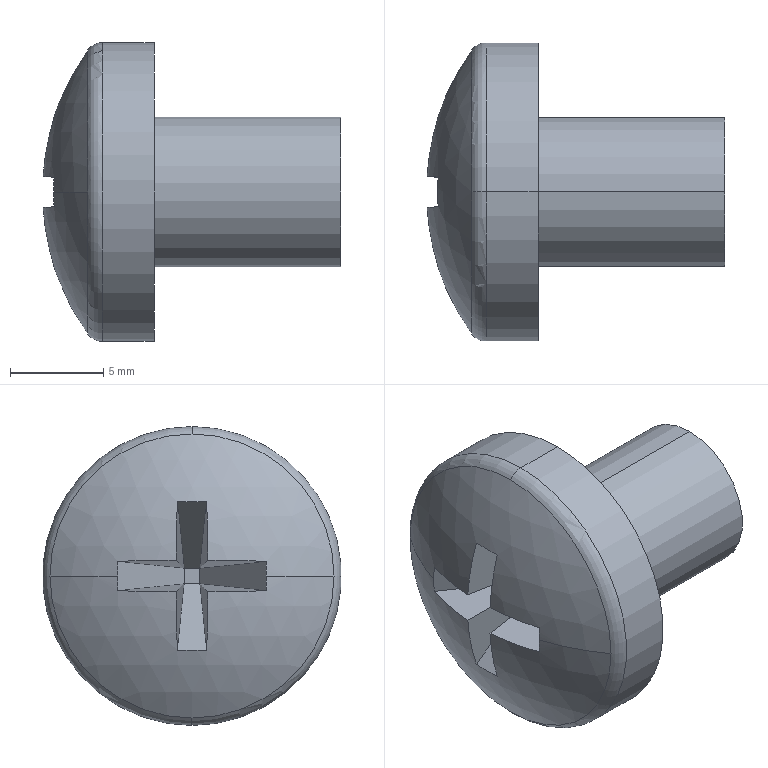Part | STEP file | pan cross head_am_B18.6.7M - M8 x 1.25 x 10 Type I Cross Recessed PHMS --10N | 1 solid | 23 faces | box 15.946 x 16 x 16 mm | volume 1390 mm3 | plane 15 | cylinder 4 | torus 2 | sphere 2 | commonest cylinder face diameters 8 x2 16 x2